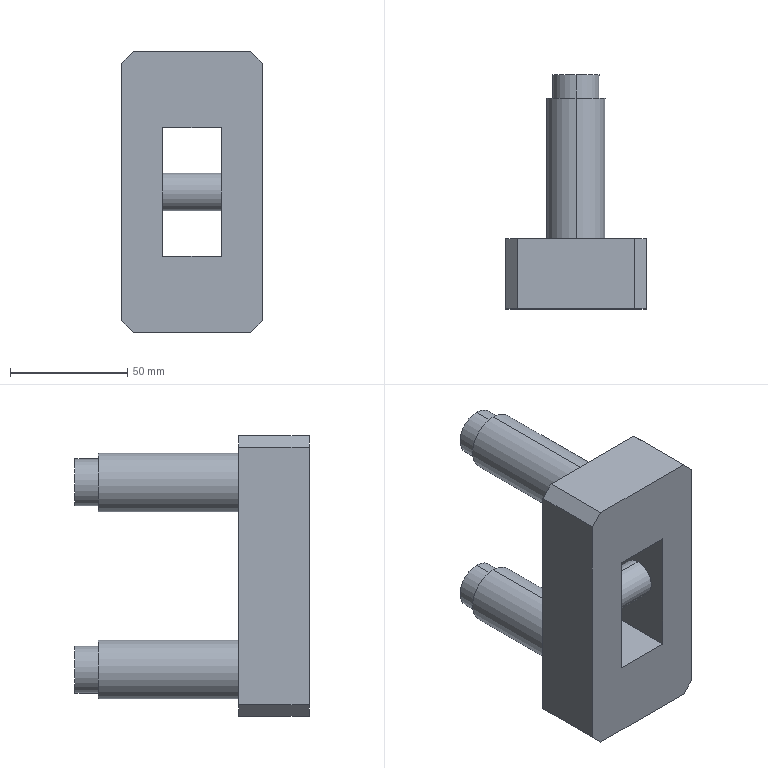Part | STEP file | PN_0012 Swing pressure plate | 3 solids | 30 faces | box 60 x 100 x 120 mm | volume 243465 mm3 | plane 20 | cylinder 10 | commonest cylinder face diameters 20 x4 25 x4 16 x2